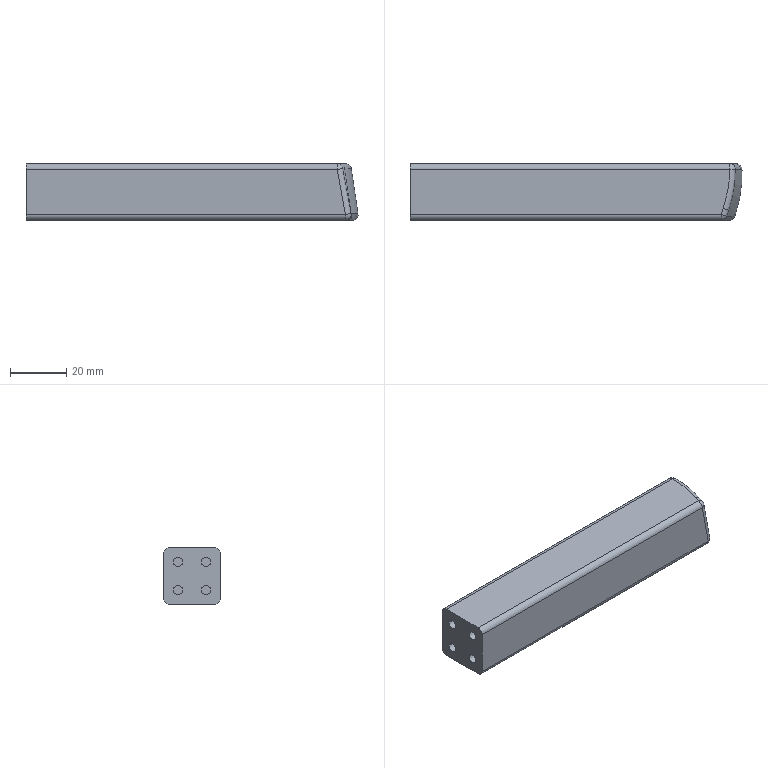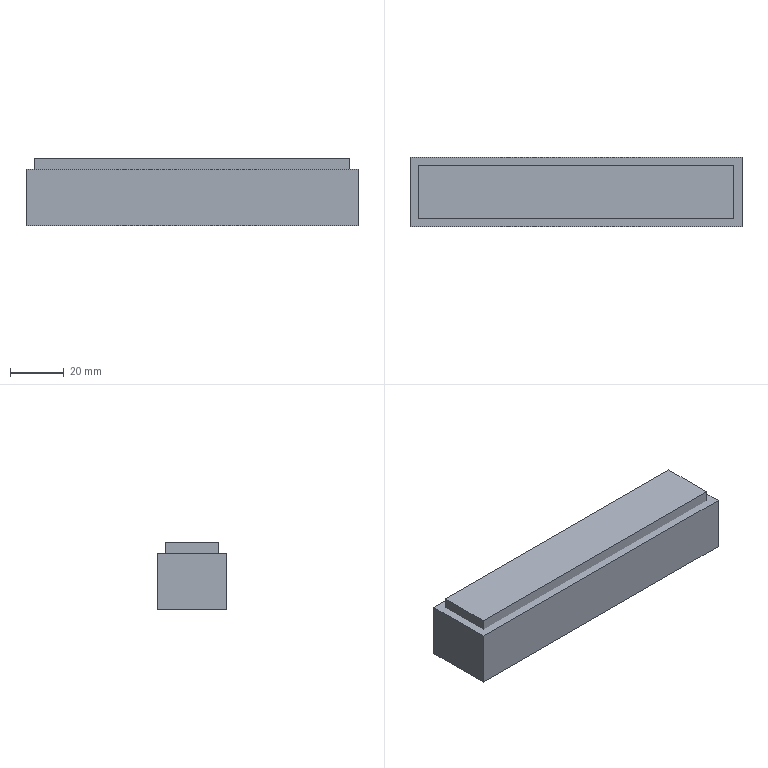CAM job | NX | 3+2 milling, drilling | part box 117.695 x 20 x 20.003 mm | stock box 123.695 x 26 x 25.003 mm
Tools:
number,name,description,diameter,corner_radius,flute_length,length,flutes
1,D63,Milling Tool-5 Parameters,63.0,0.0,50.0,75.0,2
9,D10,Milling Tool-5 Parameters,10.0,0.0,50.0,75.0,2
10,D10JING,Milling Tool-5 Parameters,10.0,0.0,50.0,75.0,2
8,D6R0.5,Milling Tool-5 Parameters,6.0,0.5,50.0,75.0,2
2,D4A45,Milling Tool-5 Parameters,4.0,0.0,2.0,2.0,2
12,3.3ZT,Drilling Tool,3.3,0.0,35.0,50.0,2
Operations:
program,operation,operation_type,tool,method,geometry_group,spindle_rpm,surface_speed,feed_per_tooth,feed_cut,feed_plunge,cut_length_mm,path_length_mm,cut_time_min,machine_time_min
1虎钳,FLOOR_WALL,VolumeBased25DMillingOperation,D63,METHOD,A,6500.0,1286.0,0.0962,1250.0,100.0,198.695,252.695,0.159,0.1644
1虎钳,ZLEVEL_PROFILE,ZLevelMilling,D10,METHOD,A,9500.0,298.0,0.1579,3000.0,1000.0,6127.194,6204.194,2.074,2.082
1虎钳,ZLEVEL_PROFILE_COPY_COPY,ZLevelMilling,D10JING,METHOD,A,9500.0,119.0,0.0632,1200.0,1000.0,311.252,408.252,0.2601,0.2698
1虎钳,ZLEVEL_PROFILE_COPY,ZLevelMilling,D6R0.5,METHOD,A,9500.0,179.0,0.1579,3000.0,1000.0,10651.866,10711.375,3.553,3.559
1虎钳,ZLEVEL_PROFILE_COPY_COPY_1,ZLevelMilling,D6R0.5,METHOD,A,9500.0,179.0,0.1579,3000.0,1000.0,5508.654,5930.905,1.845,1.887
2虎钳,FLOOR_WALL_COPY,VolumeBased25DMillingOperation,D63,METHOD,B,6500.0,1286.0,0.0962,1250.0,100.0,963.476,1960.258,0.7708,0.8705
2虎钳,ZLEVEL_PROFILE_COPY_COPY_2,ZLevelMilling,D6R0.5,METHOD,B,9500.0,179.0,0.1579,3000.0,1000.0,10865.39,10924.9,3.624,3.63
3,DRILLING_COPY,Operation,D4A45,METHOD,C,5000.0,62.0,0.025,250.0,0.0,16.0,132.321,0.064,0.0756
3,DRILLING_COPY_COPY,Operation,3.3ZT,METHOD,C,1910.0,21.0,0.0471,180.0,0.0,60.0,220.321,0.3333,0.3494